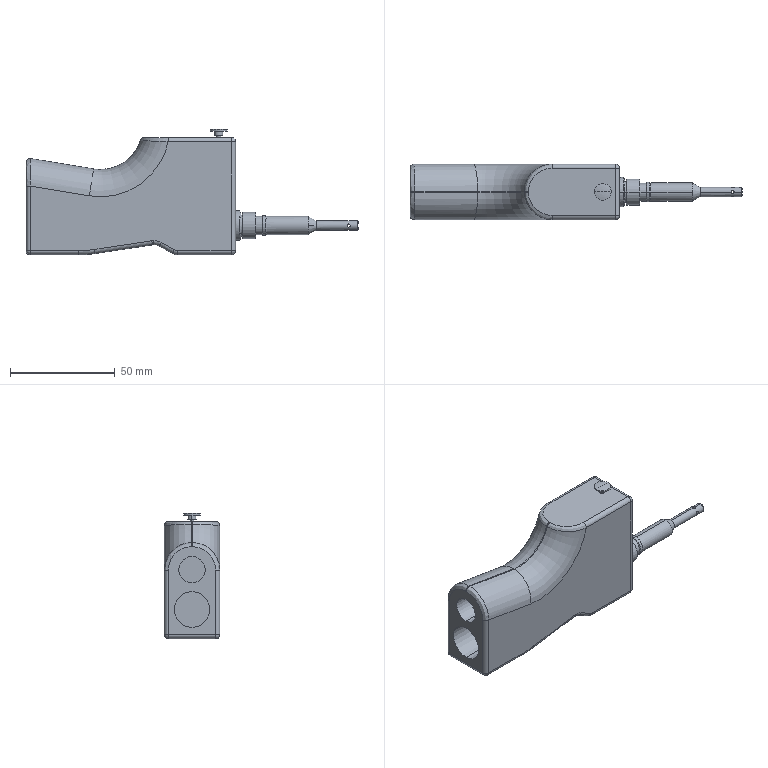Part | SolidWorks | features BaseBody 3 | 2 solids | 168 faces | box 158.45 x 26.5 x 60 mm | volume 118461 mm3 | cylinder 80 | cone 32 | plane 28 | torus 12 | spline 12 | sphere 4 | commonest cylinder face diameters 4 x21 1.5 x10 8.7 x6 10 x6 9.5 x4 12.5 x4